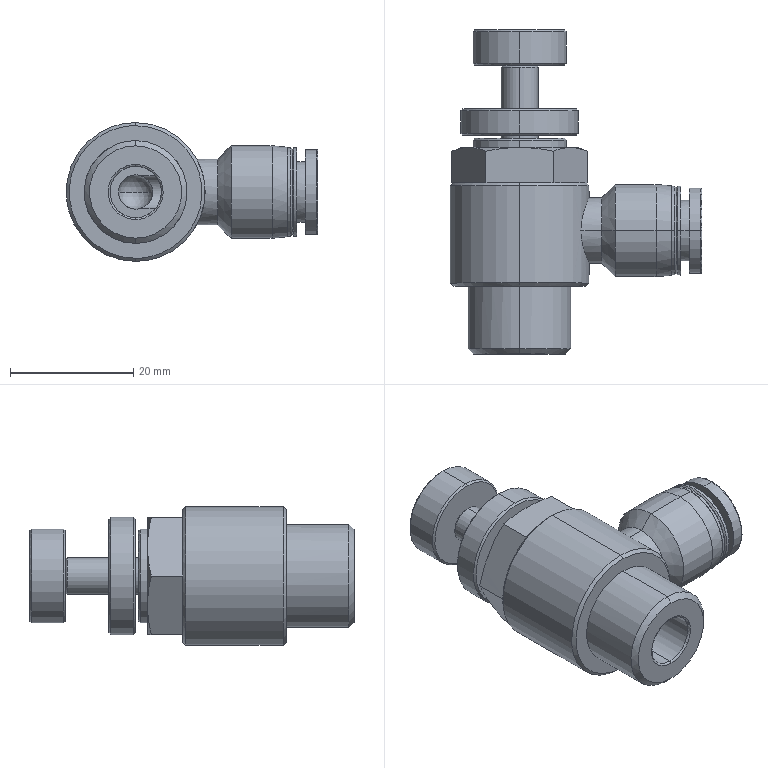Part | SolidWorks | features BaseBody 1 | 1 solid | 120 faces | box 40.75 x 52.5 x 22.5 mm | volume 13948 mm3 | plane 44 | cylinder 36 | cone 32 | torus 6 | sphere 2 | commonest cylinder face diameters 6 x4 14.4 x4 15.2 x4 5.333 x2 5.554 x2 8 x2